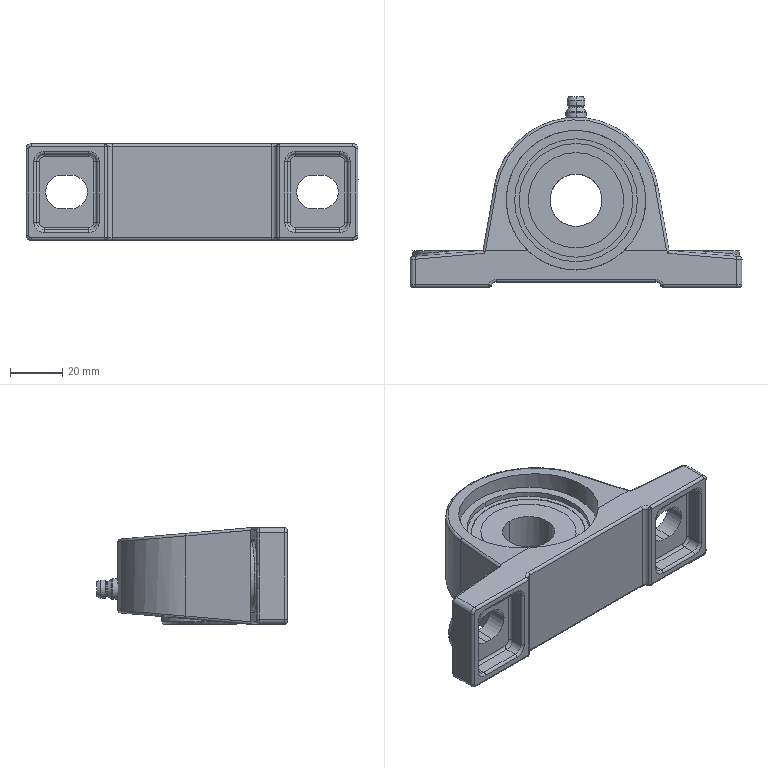Part | SolidWorks | features BaseBody 1 | 1 solid | 211 faces | box 127 x 73 x 37 mm | volume 102331 mm3 | cylinder 98 | plane 45 | torus 36 | spline 14 | cone 10 | sphere 8 | commonest cylinder face diameters 2 x46 6 x8 4 x6 13 x6 5 x4 36.5 x4